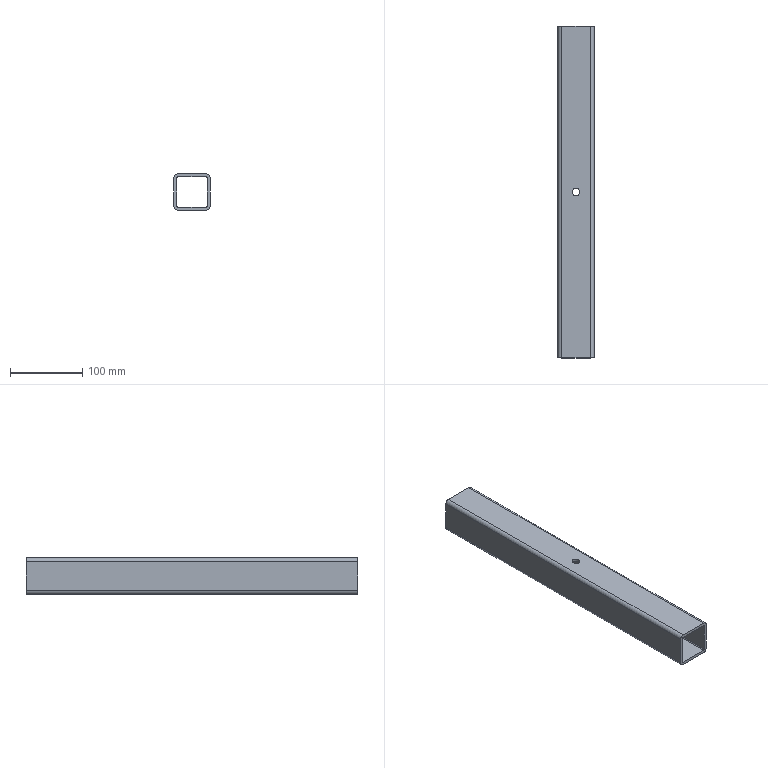Part | STEP file | 冲床-300配套压波_id1154_x_t | 1 solid | 20 faces | box 50 x 460 x 50 mm | volume 328364 mm3 | plane 10 | cylinder 10 | commonest cylinder face diameters 2 x4 10 x4 10.7 x2
STEP:
#1=CARTESIAN_POINT('',(1916.,230.,-25.));
#2=VERTEX_POINT('',#1);
#3=CARTESIAN_POINT('',(1916.,230.,-65.));
#4=VERTEX_POINT('',#3);
#5=CARTESIAN_POINT('',(1916.,230.,180.));
#6=DIRECTION('',(0.,0.,-1.));
#7=VECTOR('',#6,1.);
#8=LINE('',#5,#7);
#9=EDGE_CURVE('',#2,#4,#8,.T.);
#10=ORIENTED_EDGE('',*,*,#9,.F.);
#11=CARTESIAN_POINT('',(1915.,230.,-24.));
#12=VERTEX_POINT('',#11);
#13=CARTESIAN_POINT('',(1915.,230.,-25.));
#14=DIRECTION('',(0.,1.,0.));
#15=DIRECTION('',(-1.,0.,0.));
#16=AXIS2_PLACEMENT_3D('',#13,#14,#15);
#17=CIRCLE('',#16,1.);
#18=EDGE_CURVE('',#12,#2,#17,.T.);
#19=ORIENTED_EDGE('',*,*,#18,.F.);
#20=CARTESIAN_POINT('',(1875.,230.,-24.));
#21=VERTEX_POINT('',#20);
#22=CARTESIAN_POINT('',(3070.,230.,-24.));
#23=DIRECTION('',(1.,0.,0.));
#24=VECTOR('',#23,1.);
#25=LINE('',#22,#24);
#26=EDGE_CURVE('',#21,#12,#25,.T.);
#27=ORIENTED_EDGE('',*,*,#26,.F.);
#28=CARTESIAN_POINT('',(1874.,230.,-25.));
#29=VERTEX_POINT('',#28);
#30=CARTESIAN_POINT('',(1875.,230.,-25.));
#31=DIRECTION('',(0.,1.,0.));
#32=DIRECTION('',(-1.,0.,0.));
#33=AXIS2_PLACEMENT_3D('',#30,#31,#32);
#34=CIRCLE('',#33,1.);
#35=EDGE_CURVE('',#29,#21,#34,.T.);
#36=ORIENTED_EDGE('',*,*,#35,.F.);
#37=CARTESIAN_POINT('',(1874.,230.,-65.));
#38=VERTEX_POINT('',#37);
#39=CARTESIAN_POINT('',(1874.,230.,180.));
#40=DIRECTION('',(0.,0.,1.));
#41=VECTOR('',#40,1.);
#42=LINE('',#39,#41);
#43=EDGE_CURVE('',#38,#29,#42,.T.);
#44=ORIENTED_EDGE('',*,*,#43,.F.);
#45=CARTESIAN_POINT('',(1875.,230.,-66.));
#46=VERTEX_POINT('',#45);
#47=CARTESIAN_POINT('',(1875.,230.,-65.));
#48=DIRECTION('',(0.,1.,0.));
#49=DIRECTION('',(-1.,0.,0.));
#50=AXIS2_PLACEMENT_3D('',#47,#48,#49);
#51=CIRCLE('',#50,1.);
#52=EDGE_CURVE('',#46,#38,#51,.T.);
#53=ORIENTED_EDGE('',*,*,#52,.F.);
#54=CARTESIAN_POINT('',(1915.,230.,-66.));
#55=VERTEX_POINT('',#54);
#56=CARTESIAN_POINT('',(3070.,230.,-66.));
#57=DIRECTION('',(-1.,0.,0.));
#58=VECTOR('',#57,1.);
#59=LINE('',#56,#58);
#60=EDGE_CURVE('',#55,#46,#59,.T.);
#61=ORIENTED_EDGE('',*,*,#60,.F.);
#62=CARTESIAN_POINT('',(1915.,230.,-65.));
#63=DIRECTION('',(0.,1.,0.));
#64=DIRECTION('',(-1.,0.,0.));
#65=AXIS2_PLACEMENT_3D('',#62,#63,#64);
#66=CIRCLE('',#65,1.);
#67=EDGE_CURVE('',#4,#55,#66,.T.);
#68=ORIENTED_EDGE('',*,*,#67,.F.);
#69=EDGE_LOOP('',(#10,#19,#27,#36,#44,#53,#61,#68));
#70=FACE_BOUND('',#69,.T.);
#71=CARTESIAN_POINT('',(1920.,230.,-25.));
#72=VERTEX_POINT('',#71);
#73=CARTESIAN_POINT('',(1920.,230.,-65.));
#74=VERTEX_POINT('',#73);
#75=CARTESIAN_POINT('',(1920.,230.,-65.));
#76=DIRECTION('',(0.,0.,-1.));
#77=VECTOR('',#76,1.);
#78=LINE('',#75,#77);
#79=EDGE_CURVE('',#72,#74,#78,.T.);
#80=ORIENTED_EDGE('',*,*,#79,.T.);
#81=CARTESIAN_POINT('',(1915.,230.,-70.));
#82=VERTEX_POINT('',#81);
#83=CARTESIAN_POINT('',(1915.,230.,-65.));
#84=DIRECTION('',(0.,1.,0.));
#85=DIRECTION('',(-1.,0.,0.));
#86=AXIS2_PLACEMENT_3D('',#83,#84,#85);
#87=CIRCLE('',#86,5.);
#88=EDGE_CURVE('',#74,#82,#87,.T.);
#89=ORIENTED_EDGE('',*,*,#88,.T.);
#90=CARTESIAN_POINT('',(1875.,230.,-70.));
#91=VERTEX_POINT('',#90);
#92=CARTESIAN_POINT('',(1875.,230.,-70.));
#93=DIRECTION('',(-1.,0.,0.));
#94=VECTOR('',#93,1.);
#95=LINE('',#92,#94);
#96=EDGE_CURVE('',#82,#91,#95,.T.);
#97=ORIENTED_EDGE('',*,*,#96,.T.);
#98=CARTESIAN_POINT('',(1870.,230.,-65.));
#99=VERTEX_POINT('',#98);
#100=CARTESIAN_POINT('',(1875.,230.,-65.));
#101=DIRECTION('',(0.,1.,0.));
#102=DIRECTION('',(-1.,0.,0.));
#103=AXIS2_PLACEMENT_3D('',#100,#101,#102);
#104=CIRCLE('',#103,5.);
#105=EDGE_CURVE('',#91,#99,#104,.T.);
#106=ORIENTED_EDGE('',*,*,#105,.T.);
#107=CARTESIAN_POINT('',(1870.,230.,-25.));
#108=VERTEX_POINT('',#107);
#109=CARTESIAN_POINT('',(1870.,230.,-25.));
#110=DIRECTION('',(0.,0.,1.));
#111=VECTOR('',#110,1.);
#112=LINE('',#109,#111);
#113=EDGE_CURVE('',#99,#108,#112,.T.);
#114=ORIENTED_EDGE('',*,*,#113,.T.);
#115=CARTESIAN_POINT('',(1875.,230.,-20.));
#116=VERTEX_POINT('',#115);
#117=CARTESIAN_POINT('',(1875.,230.,-25.));
#118=DIRECTION('',(0.,1.,0.));
#119=DIRECTION('',(-1.,0.,0.));
#120=AXIS2_PLACEMENT_3D('',#117,#118,#119);
#121=CIRCLE('',#120,5.);
#122=EDGE_CURVE('',#108,#116,#121,.T.);
#123=ORIENTED_EDGE('',*,*,#122,.T.);
#124=CARTESIAN_POINT('',(1915.,230.,-20.));
#125=VERTEX_POINT('',#124);
#126=CARTESIAN_POINT('',(1915.,230.,-20.));
#127=DIRECTION('',(1.,0.,0.));
#128=VECTOR('',#127,1.);
#129=LINE('',#126,#128);
#130=EDGE_CURVE('',#116,#125,#129,.T.);
#131=ORIENTED_EDGE('',*,*,#130,.T.);
#132=CARTESIAN_POINT('',(1915.,230.,-25.));
#133=DIRECTION('',(0.,1.,0.));
#134=DIRECTION('',(-1.,0.,0.));
#135=AXIS2_PLACEMENT_3D('',#132,#133,#134);
#136=CIRCLE('',#135,5.);
#137=EDGE_CURVE('',#125,#72,#136,.T.);
#138=ORIENTED_EDGE('',*,*,#137,.T.);
#139=EDGE_LOOP('',(#80,#89,#97,#106,#114,#123,#131,#138));
#140=FACE_BOUND('',#139,.T.);
#141=CARTESIAN_POINT('',(3070.,230.,180.));
#142=DIRECTION('',(0.,1.,0.));
#143=DIRECTION('',(-1.,0.,0.));
#144=AXIS2_PLACEMENT_3D('',#141,#142,#143);
#145=PLANE('',#144);
#146=ADVANCED_FACE('',(#70,#140),#145,.T.);
#147=CARTESIAN_POINT('',(1915.,-230.,-20.));
#148=VERTEX_POINT('',#147);
#149=CARTESIAN_POINT('',(1915.,-520.,-20.));
#150=DIRECTION('',(0.,-1.,0.));
#151=VECTOR('',#150,1.);
#152=LINE('',#149,#151);
#153=EDGE_CURVE('',#125,#148,#152,.T.);
#154=ORIENTED_EDGE('',*,*,#153,.T.);
#155=CARTESIAN_POINT('',(1920.,-230.,-25.));
#156=VERTEX_POINT('',#155);
#157=CARTESIAN_POINT('',(1915.,-230.,-25.));
#158=DIRECTION('',(0.,1.,0.));
#159=DIRECTION('',(-1.,0.,0.));
#160=AXIS2_PLACEMENT_3D('',#157,#158,#159);
#161=CIRCLE('',#160,5.);
#162=EDGE_CURVE('',#148,#156,#161,.T.);
#163=ORIENTED_EDGE('',*,*,#162,.T.);
#164=CARTESIAN_POINT('',(1920.,-520.,-25.));
#165=DIRECTION('',(0.,-1.,0.));
#166=VECTOR('',#165,1.);
#167=LINE('',#164,#166);
#168=EDGE_CURVE('',#72,#156,#167,.T.);
#169=ORIENTED_EDGE('',*,*,#168,.F.);
#170=ORIENTED_EDGE('',*,*,#137,.F.);
#171=EDGE_LOOP('',(#154,#163,#169,#170));
#172=FACE_OUTER_BOUND('',#171,.T.);
#173=CARTESIAN_POINT('',(1915.,-520.,-25.));
#174=DIRECTION('',(0.,1.,0.));
#175=DIRECTION('',(-1.,0.,0.));
#176=AXIS2_PLACEMENT_3D('',#173,#174,#175);
#177=CYLINDRICAL_SURFACE('',#176,5.);
#178=ADVANCED_FACE('',(#172),#177,.T.);
#179=CARTESIAN_POINT('',(1900.35,0.,-20.));
#180=VERTEX_POINT('',#179);
#181=CARTESIAN_POINT('',(1895.,0.,-20.));
#182=DIRECTION('',(0.,0.,1.));
#183=DIRECTION('',(1.,0.,0.));
#184=AXIS2_PLACEMENT_3D('',#181,#182,#183);
#185=CIRCLE('',#184,5.35);
#186=EDGE_CURVE('',#180,#180,#185,.T.);
#187=ORIENTED_EDGE('',*,*,#186,.F.);
#188=EDGE_LOOP('',(#187));
#189=FACE_BOUND('',#188,.T.);
#190=CARTESIAN_POINT('',(1875.,-230.,-20.));
#191=VERTEX_POINT('',#190);
#192=CARTESIAN_POINT('',(1875.,-520.,-20.));
#193=DIRECTION('',(0.,-1.,0.));
#194=VECTOR('',#193,1.);
#195=LINE('',#192,#194);
#196=EDGE_CURVE('',#116,#191,#195,.T.);
#197=ORIENTED_EDGE('',*,*,#196,.T.);
#198=CARTESIAN_POINT('',(1915.,-230.,-20.));
#199=DIRECTION('',(1.,0.,0.));
#200=VECTOR('',#199,1.);
#201=LINE('',#198,#200);
#202=EDGE_CURVE('',#191,#148,#201,.T.);
#203=ORIENTED_EDGE('',*,*,#202,.T.);
#204=ORIENTED_EDGE('',*,*,#153,.F.);
#205=ORIENTED_EDGE('',*,*,#130,.F.);
#206=EDGE_LOOP('',(#197,#203,#204,#205));
#207=FACE_BOUND('',#206,.T.);
#208=CARTESIAN_POINT('',(1915.,-520.,-20.));
#209=DIRECTION('',(0.,0.,1.));
#210=DIRECTION('',(-1.,0.,0.));
#211=AXIS2_PLACEMENT_3D('',#208,#209,#210);
#212=PLANE('',#211);
#213=ADVANCED_FACE('',(#189,#207),#212,.T.);
#214=CARTESIAN_POINT('',(1870.,-230.,-25.));
#215=VERTEX_POINT('',#214);
#216=CARTESIAN_POINT('',(1870.,-520.,-25.));
#217=DIRECTION('',(0.,-1.,0.));
#218=VECTOR('',#217,1.);
#219=LINE('',#216,#218);
#220=EDGE_CURVE('',#108,#215,#219,.T.);
#221=ORIENTED_EDGE('',*,*,#220,.T.);
#222=CARTESIAN_POINT('',(1875.,-230.,-25.));
#223=DIRECTION('',(0.,1.,0.));
#224=DIRECTION('',(-1.,0.,0.));
#225=AXIS2_PLACEMENT_3D('',#222,#223,#224);
#226=CIRCLE('',#225,5.);
#227=EDGE_CURVE('',#215,#191,#226,.T.);
#228=ORIENTED_EDGE('',*,*,#227,.T.);
#229=ORIENTED_EDGE('',*,*,#196,.F.);
#230=ORIENTED_EDGE('',*,*,#122,.F.);
#231=EDGE_LOOP('',(#221,#228,#229,#230));
#232=FACE_OUTER_BOUND('',#231,.T.);
#233=CARTESIAN_POINT('',(1875.,-520.,-25.));
#234=DIRECTION('',(0.,1.,0.));
#235=DIRECTION('',(-1.,0.,0.));
#236=AXIS2_PLACEMENT_3D('',#233,#234,#235);
#237=CYLINDRICAL_SURFACE('',#236,5.);
#238=ADVANCED_FACE('',(#232),#237,.T.);
#239=CARTESIAN_POINT('',(1870.,-230.,-65.));
#240=VERTEX_POINT('',#239);
#241=CARTESIAN_POINT('',(1870.,-520.,-65.));
#242=DIRECTION('',(0.,-1.,0.));
#243=VECTOR('',#242,1.);
#244=LINE('',#241,#243);
#245=EDGE_CURVE('',#99,#240,#244,.T.);
#246=ORIENTED_EDGE('',*,*,#245,.T.);
#247=CARTESIAN_POINT('',(1870.,-230.,-740.));
#248=DIRECTION('',(0.,0.,1.));
#249=VECTOR('',#248,1.);
#250=LINE('',#247,#249);
#251=EDGE_CURVE('',#240,#215,#250,.T.);
#252=ORIENTED_EDGE('',*,*,#251,.T.);
#253=ORIENTED_EDGE('',*,*,#220,.F.);
#254=ORIENTED_EDGE('',*,*,#113,.F.);
#255=EDGE_LOOP('',(#246,#252,#253,#254));
#256=FACE_OUTER_BOUND('',#255,.T.);
#257=CARTESIAN_POINT('',(1870.,-520.,-25.));
#258=DIRECTION('',(-1.,0.,0.));
#259=DIRECTION('',(0.,-1.,0.));
#260=AXIS2_PLACEMENT_3D('',#257,#258,#259);
#261=PLANE('',#260);
#262=ADVANCED_FACE('',(#256),#261,.T.);
#263=CARTESIAN_POINT('',(1875.,-230.,-70.));
#264=VERTEX_POINT('',#263);
#265=CARTESIAN_POINT('',(1875.,-520.,-70.));
#266=DIRECTION('',(0.,-1.,0.));
#267=VECTOR('',#266,1.);
#268=LINE('',#265,#267);
#269=EDGE_CURVE('',#91,#264,#268,.T.);
#270=ORIENTED_EDGE('',*,*,#269,.T.);
#271=CARTESIAN_POINT('',(1875.,-230.,-65.));
#272=DIRECTION('',(0.,1.,0.));
#273=DIRECTION('',(-1.,0.,0.));
#274=AXIS2_PLACEMENT_3D('',#271,#272,#273);
#275=CIRCLE('',#274,5.);
#276=EDGE_CURVE('',#264,#240,#275,.T.);
#277=ORIENTED_EDGE('',*,*,#276,.T.);
#278=ORIENTED_EDGE('',*,*,#245,.F.);
#279=ORIENTED_EDGE('',*,*,#105,.F.);
#280=EDGE_LOOP('',(#270,#277,#278,#279));
#281=FACE_OUTER_BOUND('',#280,.T.);
#282=CARTESIAN_POINT('',(1875.,-520.,-65.));
#283=DIRECTION('',(0.,1.,0.));
#284=DIRECTION('',(-1.,0.,0.));
#285=AXIS2_PLACEMENT_3D('',#282,#283,#284);
#286=CYLINDRICAL_SURFACE('',#285,5.);
#287=ADVANCED_FACE('',(#281),#286,.T.);
#288=CARTESIAN_POINT('',(1916.,-230.,-65.));
#289=VERTEX_POINT('',#288);
#290=CARTESIAN_POINT('',(1915.,-230.,-66.));
#291=VERTEX_POINT('',#290);
#292=CARTESIAN_POINT('',(1915.,-230.,-65.));
#293=DIRECTION('',(0.,1.,0.));
#294=DIRECTION('',(-1.,0.,0.));
#295=AXIS2_PLACEMENT_3D('',#292,#293,#294);
#296=CIRCLE('',#295,1.);
#297=EDGE_CURVE('',#289,#291,#296,.T.);
#298=ORIENTED_EDGE('',*,*,#297,.T.);
#299=CARTESIAN_POINT('',(1875.,-230.,-66.));
#300=VERTEX_POINT('',#299);
#301=CARTESIAN_POINT('',(1915.,-230.,-66.));
#302=DIRECTION('',(-1.,0.,0.));
#303=VECTOR('',#302,1.);
#304=LINE('',#301,#303);
#305=EDGE_CURVE('',#291,#300,#304,.T.);
#306=ORIENTED_EDGE('',*,*,#305,.T.);
#307=CARTESIAN_POINT('',(1874.,-230.,-65.));
#308=VERTEX_POINT('',#307);
#309=CARTESIAN_POINT('',(1875.,-230.,-65.));
#310=DIRECTION('',(0.,1.,0.));
#311=DIRECTION('',(-1.,0.,0.));
#312=AXIS2_PLACEMENT_3D('',#309,#310,#311);
#313=CIRCLE('',#312,1.);
#314=EDGE_CURVE('',#300,#308,#313,.T.);
#315=ORIENTED_EDGE('',*,*,#314,.T.);
#316=CARTESIAN_POINT('',(1874.,-230.,-25.));
#317=VERTEX_POINT('',#316);
#318=CARTESIAN_POINT('',(1874.,-230.,-740.));
#319=DIRECTION('',(0.,0.,1.));
#320=VECTOR('',#319,1.);
#321=LINE('',#318,#320);
#322=EDGE_CURVE('',#308,#317,#321,.T.);
#323=ORIENTED_EDGE('',*,*,#322,.T.);
#324=CARTESIAN_POINT('',(1875.,-230.,-24.));
#325=VERTEX_POINT('',#324);
#326=CARTESIAN_POINT('',(1875.,-230.,-25.));
#327=DIRECTION('',(0.,1.,0.));
#328=DIRECTION('',(-1.,0.,0.));
#329=AXIS2_PLACEMENT_3D('',#326,#327,#328);
#330=CIRCLE('',#329,1.);
#331=EDGE_CURVE('',#317,#325,#330,.T.);
#332=ORIENTED_EDGE('',*,*,#331,.T.);
#333=CARTESIAN_POINT('',(1915.,-230.,-24.));
#334=VERTEX_POINT('',#333);
#335=CARTESIAN_POINT('',(1915.,-230.,-24.));
#336=DIRECTION('',(1.,0.,0.));
#337=VECTOR('',#336,1.);
#338=LINE('',#335,#337);
#339=EDGE_CURVE('',#325,#334,#338,.T.);
#340=ORIENTED_EDGE('',*,*,#339,.T.);
#341=CARTESIAN_POINT('',(1916.,-230.,-25.));
#342=VERTEX_POINT('',#341);
#343=CARTESIAN_POINT('',(1915.,-230.,-25.));
#344=DIRECTION('',(0.,1.,0.));
#345=DIRECTION('',(-1.,0.,0.));
#346=AXIS2_PLACEMENT_3D('',#343,#344,#345);
#347=CIRCLE('',#346,1.);
#348=EDGE_CURVE('',#334,#342,#347,.T.);
#349=ORIENTED_EDGE('',*,*,#348,.T.);
#350=CARTESIAN_POINT('',(1916.,-230.,-740.));
#351=DIRECTION('',(0.,0.,-1.));
#352=VECTOR('',#351,1.);
#353=LINE('',#350,#352);
#354=EDGE_CURVE('',#342,#289,#353,.T.);
#355=ORIENTED_EDGE('',*,*,#354,.T.);
#356=EDGE_LOOP('',(#298,#306,#315,#323,#332,#340,#349,#355));
#357=FACE_BOUND('',#356,.T.);
#358=CARTESIAN_POINT('',(1920.,-230.,-65.));
#359=VERTEX_POINT('',#358);
#360=CARTESIAN_POINT('',(1920.,-230.,-740.));
#361=DIRECTION('',(0.,0.,-1.));
#362=VECTOR('',#361,1.);
#363=LINE('',#360,#362);
#364=EDGE_CURVE('',#156,#359,#363,.T.);
#365=ORIENTED_EDGE('',*,*,#364,.F.);
#366=ORIENTED_EDGE('',*,*,#162,.F.);
#367=ORIENTED_EDGE('',*,*,#202,.F.);
#368=ORIENTED_EDGE('',*,*,#227,.F.);
#369=ORIENTED_EDGE('',*,*,#251,.F.);
#370=ORIENTED_EDGE('',*,*,#276,.F.);
#371=CARTESIAN_POINT('',(1915.,-230.,-70.));
#372=VERTEX_POINT('',#371);
#373=CARTESIAN_POINT('',(1915.,-230.,-70.));
#374=DIRECTION('',(-1.,0.,0.));
#375=VECTOR('',#374,1.);
#376=LINE('',#373,#375);
#377=EDGE_CURVE('',#372,#264,#376,.T.);
#378=ORIENTED_EDGE('',*,*,#377,.F.);
#379=CARTESIAN_POINT('',(1915.,-230.,-65.));
#380=DIRECTION('',(0.,1.,0.));
#381=DIRECTION('',(-1.,0.,0.));
#382=AXIS2_PLACEMENT_3D('',#379,#380,#381);
#383=CIRCLE('',#382,5.);
#384=EDGE_CURVE('',#359,#372,#383,.T.);
#385=ORIENTED_EDGE('',*,*,#384,.F.);
#386=EDGE_LOOP('',(#365,#366,#367,#368,#369,#370,#378,#385));
#387=FACE_BOUND('',#386,.T.);
#388=CARTESIAN_POINT('',(1915.,-230.,-740.));
#389=DIRECTION('',(0.,1.,0.));
#390=DIRECTION('',(-1.,0.,0.));
#391=AXIS2_PLACEMENT_3D('',#388,#389,#390);
#392=PLANE('',#391);
#393=ADVANCED_FACE('',(#357,#387),#392,.F.);
#394=CARTESIAN_POINT('',(1889.65,0.,-70.));
#395=VERTEX_POINT('',#394);
#396=CARTESIAN_POINT('',(1895.,0.,-70.));
#397=DIRECTION('',(0.,0.,-1.));
#398=DIRECTION('',(-1.,0.,0.));
#399=AXIS2_PLACEMENT_3D('',#396,#397,#398);
#400=CIRCLE('',#399,5.35);
#401=EDGE_CURVE('',#395,#395,#400,.T.);
#402=ORIENTED_EDGE('',*,*,#401,.F.);
#403=EDGE_LOOP('',(#402));
#404=FACE_BOUND('',#403,.T.);
#405=CARTESIAN_POINT('',(1915.,-520.,-70.));
#406=DIRECTION('',(0.,-1.,0.));
#407=VECTOR('',#406,1.);
#408=LINE('',#405,#407);
#409=EDGE_CURVE('',#82,#372,#408,.T.);
#410=ORIENTED_EDGE('',*,*,#409,.T.);
#411=ORIENTED_EDGE('',*,*,#377,.T.);
#412=ORIENTED_EDGE('',*,*,#269,.F.);
#413=ORIENTED_EDGE('',*,*,#96,.F.);
#414=EDGE_LOOP('',(#410,#411,#412,#413));
#415=FACE_BOUND('',#414,.T.);
#416=CARTESIAN_POINT('',(1875.,-520.,-70.));
#417=DIRECTION('',(0.,0.,-1.));
#418=DIRECTION('',(1.,0.,0.));
#419=AXIS2_PLACEMENT_3D('',#416,#417,#418);
#420=PLANE('',#419);
#421=ADVANCED_FACE('',(#404,#415),#420,.T.);
#422=ORIENTED_EDGE('',*,*,#168,.T.);
#423=ORIENTED_EDGE('',*,*,#364,.T.);
#424=CARTESIAN_POINT('',(1920.,-520.,-65.));
#425=DIRECTION('',(0.,-1.,0.));
#426=VECTOR('',#425,1.);
#427=LINE('',#424,#426);
#428=EDGE_CURVE('',#74,#359,#427,.T.);
#429=ORIENTED_EDGE('',*,*,#428,.F.);
#430=ORIENTED_EDGE('',*,*,#79,.F.);
#431=EDGE_LOOP('',(#422,#423,#429,#430));
#432=FACE_OUTER_BOUND('',#431,.T.);
#433=CARTESIAN_POINT('',(1920.,-520.,-65.));
#434=DIRECTION('',(1.,0.,0.));
#435=DIRECTION('',(0.,1.,0.));
#436=AXIS2_PLACEMENT_3D('',#433,#434,#435);
#437=PLANE('',#436);
#438=ADVANCED_FACE('',(#432),#437,.T.);
#439=ORIENTED_EDGE('',*,*,#428,.T.);
#440=ORIENTED_EDGE('',*,*,#384,.T.);
#441=ORIENTED_EDGE('',*,*,#409,.F.);
#442=ORIENTED_EDGE('',*,*,#88,.F.);
#443=EDGE_LOOP('',(#439,#440,#441,#442));
#444=FACE_OUTER_BOUND('',#443,.T.);
#445=CARTESIAN_POINT('',(1915.,-520.,-65.));
#446=DIRECTION('',(0.,1.,0.));
#447=DIRECTION('',(-1.,0.,0.));
#448=AXIS2_PLACEMENT_3D('',#445,#446,#447);
#449=CYLINDRICAL_SURFACE('',#448,5.);
#450=ADVANCED_FACE('',(#444),#449,.T.);
#451=CARTESIAN_POINT('',(1915.,-520.,-24.));
#452=DIRECTION('',(0.,-1.,0.));
#453=VECTOR('',#452,1.);
#454=LINE('',#451,#453);
#455=EDGE_CURVE('',#12,#334,#454,.T.);
#456=ORIENTED_EDGE('',*,*,#455,.F.);
#457=ORIENTED_EDGE('',*,*,#18,.T.);
#458=CARTESIAN_POINT('',(1916.,-520.,-25.));
#459=DIRECTION('',(0.,-1.,0.));
#460=VECTOR('',#459,1.);
#461=LINE('',#458,#460);
#462=EDGE_CURVE('',#2,#342,#461,.T.);
#463=ORIENTED_EDGE('',*,*,#462,.T.);
#464=ORIENTED_EDGE('',*,*,#348,.F.);
#465=EDGE_LOOP('',(#456,#457,#463,#464));
#466=FACE_OUTER_BOUND('',#465,.T.);
#467=CARTESIAN_POINT('',(1915.,-520.,-25.));
#468=DIRECTION('',(0.,1.,0.));
#469=DIRECTION('',(-1.,0.,0.));
#470=AXIS2_PLACEMENT_3D('',#467,#468,#469);
#471=CYLINDRICAL_SURFACE('',#470,1.);
#472=ADVANCED_FACE('',(#466),#471,.F.);
#473=CARTESIAN_POINT('',(1900.35,0.,-24.));
#474=VERTEX_POINT('',#473);
#475=CARTESIAN_POINT('',(1895.,0.,-24.));
#476=DIRECTION('',(0.,0.,1.));
#477=DIRECTION('',(1.,0.,0.));
#478=AXIS2_PLACEMENT_3D('',#475,#476,#477);
#479=CIRCLE('',#478,5.35);
#480=EDGE_CURVE('',#474,#474,#479,.T.);
#481=ORIENTED_EDGE('',*,*,#480,.T.);
#482=EDGE_LOOP('',(#481));
#483=FACE_BOUND('',#482,.T.);
#484=CARTESIAN_POINT('',(1875.,-520.,-24.));
#485=DIRECTION('',(0.,-1.,0.));
#486=VECTOR('',#485,1.);
#487=LINE('',#484,#486);
#488=EDGE_CURVE('',#21,#325,#487,.T.);
#489=ORIENTED_EDGE('',*,*,#488,.F.);
#490=ORIENTED_EDGE('',*,*,#26,.T.);
#491=ORIENTED_EDGE('',*,*,#455,.T.);
#492=ORIENTED_EDGE('',*,*,#339,.F.);
#493=EDGE_LOOP('',(#489,#490,#491,#492));
#494=FACE_BOUND('',#493,.T.);
#495=CARTESIAN_POINT('',(1915.,-520.,-24.));
#496=DIRECTION('',(0.,0.,1.));
#497=DIRECTION('',(-1.,0.,0.));
#498=AXIS2_PLACEMENT_3D('',#495,#496,#497);
#499=PLANE('',#498);
#500=ADVANCED_FACE('',(#483,#494),#499,.F.);
#501=CARTESIAN_POINT('',(1874.,-520.,-25.));
#502=DIRECTION('',(0.,-1.,0.));
#503=VECTOR('',#502,1.);
#504=LINE('',#501,#503);
#505=EDGE_CURVE('',#29,#317,#504,.T.);
#506=ORIENTED_EDGE('',*,*,#505,.F.);
#507=ORIENTED_EDGE('',*,*,#35,.T.);
#508=ORIENTED_EDGE('',*,*,#488,.T.);
#509=ORIENTED_EDGE('',*,*,#331,.F.);
#510=EDGE_LOOP('',(#506,#507,#508,#509));
#511=FACE_OUTER_BOUND('',#510,.T.);
#512=CARTESIAN_POINT('',(1875.,-520.,-25.));
#513=DIRECTION('',(0.,1.,0.));
#514=DIRECTION('',(-1.,0.,0.));
#515=AXIS2_PLACEMENT_3D('',#512,#513,#514);
#516=CYLINDRICAL_SURFACE('',#515,1.);
#517=ADVANCED_FACE('',(#511),#516,.F.);
#518=CARTESIAN_POINT('',(1874.,-520.,-65.));
#519=DIRECTION('',(0.,-1.,0.));
#520=VECTOR('',#519,1.);
#521=LINE('',#518,#520);
#522=EDGE_CURVE('',#38,#308,#521,.T.);
#523=ORIENTED_EDGE('',*,*,#522,.F.);
#524=ORIENTED_EDGE('',*,*,#43,.T.);
#525=ORIENTED_EDGE('',*,*,#505,.T.);
#526=ORIENTED_EDGE('',*,*,#322,.F.);
#527=EDGE_LOOP('',(#523,#524,#525,#526));
#528=FACE_OUTER_BOUND('',#527,.T.);
#529=CARTESIAN_POINT('',(1874.,-520.,-25.));
#530=DIRECTION('',(-1.,0.,0.));
#531=DIRECTION('',(0.,-1.,0.));
#532=AXIS2_PLACEMENT_3D('',#529,#530,#531);
#533=PLANE('',#532);
#534=ADVANCED_FACE('',(#528),#533,.F.);
#535=CARTESIAN_POINT('',(1875.,-520.,-66.));
#536=DIRECTION('',(0.,-1.,0.));
#537=VECTOR('',#536,1.);
#538=LINE('',#535,#537);
#539=EDGE_CURVE('',#46,#300,#538,.T.);
#540=ORIENTED_EDGE('',*,*,#539,.F.);
#541=ORIENTED_EDGE('',*,*,#52,.T.);
#542=ORIENTED_EDGE('',*,*,#522,.T.);
#543=ORIENTED_EDGE('',*,*,#314,.F.);
#544=EDGE_LOOP('',(#540,#541,#542,#543));
#545=FACE_OUTER_BOUND('',#544,.T.);
#546=CARTESIAN_POINT('',(1875.,-520.,-65.));
#547=DIRECTION('',(0.,1.,0.));
#548=DIRECTION('',(-1.,0.,0.));
#549=AXIS2_PLACEMENT_3D('',#546,#547,#548);
#550=CYLINDRICAL_SURFACE('',#549,1.);
#551=ADVANCED_FACE('',(#545),#550,.F.);
#552=CARTESIAN_POINT('',(1889.65,0.,-66.));
#553=VERTEX_POINT('',#552);
#554=CARTESIAN_POINT('',(1895.,0.,-66.));
#555=DIRECTION('',(0.,0.,-1.));
#556=DIRECTION('',(-1.,0.,0.));
#557=AXIS2_PLACEMENT_3D('',#554,#555,#556);
#558=CIRCLE('',#557,5.35);
#559=EDGE_CURVE('',#553,#553,#558,.T.);
#560=ORIENTED_EDGE('',*,*,#559,.T.);
#561=EDGE_LOOP('',(#560));
#562=FACE_BOUND('',#561,.T.);
#563=CARTESIAN_POINT('',(1915.,-520.,-66.));
#564=DIRECTION('',(0.,-1.,0.));
#565=VECTOR('',#564,1.);
#566=LINE('',#563,#565);
#567=EDGE_CURVE('',#55,#291,#566,.T.);
#568=ORIENTED_EDGE('',*,*,#567,.F.);
#569=ORIENTED_EDGE('',*,*,#60,.T.);
#570=ORIENTED_EDGE('',*,*,#539,.T.);
#571=ORIENTED_EDGE('',*,*,#305,.F.);
#572=EDGE_LOOP('',(#568,#569,#570,#571));
#573=FACE_BOUND('',#572,.T.);
#574=CARTESIAN_POINT('',(1875.,-520.,-66.));
#575=DIRECTION('',(0.,0.,-1.));
#576=DIRECTION('',(1.,0.,0.));
#577=AXIS2_PLACEMENT_3D('',#574,#575,#576);
#578=PLANE('',#577);
#579=ADVANCED_FACE('',(#562,#573),#578,.F.);
#580=ORIENTED_EDGE('',*,*,#462,.F.);
#581=ORIENTED_EDGE('',*,*,#9,.T.);
#582=CARTESIAN_POINT('',(1916.,-520.,-65.));
#583=DIRECTION('',(0.,-1.,0.));
#584=VECTOR('',#583,1.);
#585=LINE('',#582,#584);
#586=EDGE_CURVE('',#4,#289,#585,.T.);
#587=ORIENTED_EDGE('',*,*,#586,.T.);
#588=ORIENTED_EDGE('',*,*,#354,.F.);
#589=EDGE_LOOP('',(#580,#581,#587,#588));
#590=FACE_OUTER_BOUND('',#589,.T.);
#591=CARTESIAN_POINT('',(1916.,-520.,-65.));
#592=DIRECTION('',(1.,0.,0.));
#593=DIRECTION('',(0.,1.,0.));
#594=AXIS2_PLACEMENT_3D('',#591,#592,#593);
#595=PLANE('',#594);
#596=ADVANCED_FACE('',(#590),#595,.F.);
#597=ORIENTED_EDGE('',*,*,#586,.F.);
#598=ORIENTED_EDGE('',*,*,#67,.T.);
#599=ORIENTED_EDGE('',*,*,#567,.T.);
#600=ORIENTED_EDGE('',*,*,#297,.F.);
#601=EDGE_LOOP('',(#597,#598,#599,#600));
#602=FACE_OUTER_BOUND('',#601,.T.);
#603=CARTESIAN_POINT('',(1915.,-520.,-65.));
#604=DIRECTION('',(0.,1.,0.));
#605=DIRECTION('',(-1.,0.,0.));
#606=AXIS2_PLACEMENT_3D('',#603,#604,#605);
#607=CYLINDRICAL_SURFACE('',#606,1.);
#608=ADVANCED_FACE('',(#602),#607,.F.);
#609=ORIENTED_EDGE('',*,*,#401,.T.);
#610=EDGE_LOOP('',(#609));
#611=FACE_BOUND('',#610,.T.);
#612=ORIENTED_EDGE('',*,*,#559,.F.);
#613=EDGE_LOOP('',(#612));
#614=FACE_BOUND('',#613,.T.);
#615=CARTESIAN_POINT('',(1895.,0.,83.));
#616=DIRECTION('',(0.,0.,-1.));
#617=DIRECTION('',(-1.,0.,0.));
#618=AXIS2_PLACEMENT_3D('',#615,#616,#617);
#619=CYLINDRICAL_SURFACE('',#618,5.35);
#620=ADVANCED_FACE('',(#611,#614),#619,.F.);
#621=ORIENTED_EDGE('',*,*,#186,.T.);
#622=EDGE_LOOP('',(#621));
#623=FACE_BOUND('',#622,.T.);
#624=ORIENTED_EDGE('',*,*,#480,.F.);
#625=EDGE_LOOP('',(#624));
#626=FACE_BOUND('',#625,.T.);
#627=CARTESIAN_POINT('',(1895.,0.,83.));
#628=DIRECTION('',(0.,0.,-1.));
#629=DIRECTION('',(-1.,0.,0.));
#630=AXIS2_PLACEMENT_3D('',#627,#628,#629);
#631=CYLINDRICAL_SURFACE('',#630,5.35);
#632=ADVANCED_FACE('',(#623,#626),#631,.F.);
#633=CLOSED_SHELL('',(#146,#178,#213,#238,#262,#287,#393,#421,#438,#450,#472,#500,#517,#534,#551,#579,#596,#608,#620,#632));
#634=MANIFOLD_SOLID_BREP('',#633);
#635=(LENGTH_UNIT()NAMED_UNIT(*)SI_UNIT(.MILLI.,.METRE.));
#636=UNCERTAINTY_MEASURE_WITH_UNIT(LENGTH_MEASURE(0.00002),#635,'','');
#637=(NAMED_UNIT(*)PLANE_ANGLE_UNIT()SI_UNIT($,.RADIAN.));
#638=PLANE_ANGLE_MEASURE_WITH_UNIT(PLANE_ANGLE_MEASURE(0.01745),#637);
#639=DIMENSIONAL_EXPONENTS(0.,0.,0.,0.,0.,0.,0.);
#640=(CONVERSION_BASED_UNIT('DEGREE',#638)NAMED_UNIT(#639)PLANE_ANGLE_UNIT());
#641=(NAMED_UNIT(*)SI_UNIT($,.STERADIAN.)SOLID_ANGLE_UNIT());
#642=(GEOMETRIC_REPRESENTATION_CONTEXT(3)GLOBAL_UNCERTAINTY_ASSIGNED_CONTEXT((#636))GLOBAL_UNIT_ASSIGNED_CONTEXT((#635,#640,#641))REPRESENTATION_CONTEXT('',''));
#643=ADVANCED_BREP_SHAPE_REPRESENTATION('',(#634),#642);